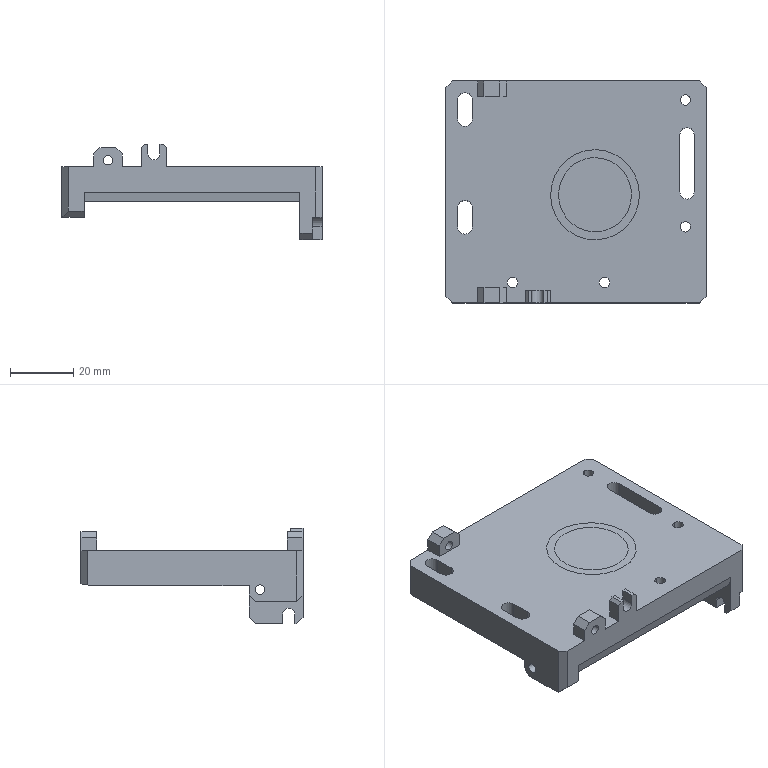NC program | NX | posted with a generic post | part box 82 x 70 x 30 mm
Whole program:
N10 G17 G21 G94 G90
(HOLE_MILLING , TOOL : D10)
N12 T10 M6
N14 G54
N16 G17 G0 G90 X34.989 Y6. B0. C0. S9500 M3
N18 G43 Z50. H10
N20 Z-1.904
N22 G94 G3 X37.177 Y8.188 R2.188 F1500.
N24 X34.989 Y10.375 R2.188
N26 X34.989 Y10.375 Z-2.404 I0. J-4.375
N28 X34.989 Y10.375 Z-2.904 I0. J-4.375
N30 X34.989 Y10.375 Z-3.404 I0. J-4.375
N32 X34.989 Y10.375 Z-3.904 I0. J-4.375
N34 X34.989 Y10.375 Z-4.404 I0. J-4.375
N36 X34.989 Y10.375 Z-4.904 I0. J-4.375
N38 X34.989 Y10.375 Z-5.404 I0. J-4.375
N40 X34.989 Y10.375 Z-5.904 I0. J-4.375
N42 X34.989 Y10.375 Z-6.404 I0. J-4.375
N44 X34.989 Y10.375 Z-6.904 I0. J-4.375
N46 X34.989 Y10.375 Z-7.404 I0. J-4.375
N48 X34.989 Y10.375 Z-7.904 I0. J-4.375
N50 X34.989 Y10.375 Z-8.404 I0. J-4.375
N52 X34.989 Y10.375 Z-8.904 I0. J-4.375
N54 X34.989 Y10.375 Z-9.404 I0. J-4.375
N56 X34.989 Y10.375 Z-9.904 I0. J-4.375
N58 X34.989 Y10.375 Z-10.404 I0. J-4.375
N60 X34.989 Y10.375 Z-10.904 I0. J-4.375
N62 X34.989 Y10.375 Z-11.404 I0. J-4.375
N64 X34.989 Y10.375 Z-11.904 I0. J-4.375
N66 X30.687 Y6.792 Z-12.015 R4.375
N68 X34.197 Y1.697 R4.375
N70 X30.687 Y6.792 R-4.375
N72 X32.442 Y4.245 R2.188
N74 X34.989 Y6. R2.188
N76 G0 Z-1.904
N78 G3 X39.364 Y10.375 R4.375
N80 X34.989 Y14.75 R4.375
N82 X34.989 Y14.75 Z-2.404 I0. J-8.75
N84 X34.989 Y14.75 Z-2.904 I0. J-8.75
N86 X34.989 Y14.75 Z-3.404 I0. J-8.75
N88 X34.989 Y14.75 Z-3.904 I0. J-8.75
N90 X34.989 Y14.75 Z-4.404 I0. J-8.75
N92 X34.989 Y14.75 Z-4.904 I0. J-8.75
N94 X34.989 Y14.75 Z-5.404 I0. J-8.75
N96 X34.989 Y14.75 Z-5.904 I0. J-8.75
N98 X34.989 Y14.75 Z-6.404 I0. J-8.75
N100 X34.989 Y14.75 Z-6.904 I0. J-8.75
N102 X34.989 Y14.75 Z-7.404 I0. J-8.75
N104 X34.989 Y14.75 Z-7.904 I0. J-8.75
N106 X34.989 Y14.75 Z-8.404 I0. J-8.75
N108 X34.989 Y14.75 Z-8.904 I0. J-8.75
N110 X34.989 Y14.75 Z-9.404 I0. J-8.75
N112 X34.989 Y14.75 Z-9.904 I0. J-8.75
N114 X34.989 Y14.75 Z-10.404 I0. J-8.75
N116 X34.989 Y14.75 Z-10.904 I0. J-8.75
N118 X34.989 Y14.75 Z-11.404 I0. J-8.75
N120 X34.989 Y14.75 Z-11.904 I0. J-8.75
N122 X26.384 Y7.584 Z-12.015 R8.75
N124 X33.405 Y-2.605 R8.75
N126 X26.384 Y7.584 R-8.75
N128 X29.894 Y2.49 R4.375
N130 X34.989 Y6. R4.375
N132 G0 Z50.
(HOLE_MILLING_COPY , TOOL : D10)
N134 Z-11.015
N136 G3 X36.864 Y7.875 R1.875
N138 X34.989 Y9.75 R1.875
N140 X34.989 Y9.75 Z-11.515 I0. J-3.75
N142 X34.989 Y9.75 Z-12.015 I0. J-3.75
N144 X34.989 Y9.75 Z-12.515 I0. J-3.75
N146 X34.989 Y9.75 Z-13.015 I0. J-3.75
N148 X34.989 Y9.75 Z-13.515 I0. J-3.75
N150 X31.239 Y6. R3.75
N152 X34.989 Y9.75 R-3.75
N154 X33.114 Y7.875 R1.875
N156 X34.989 Y6. R1.875
N158 G0 Z-11.015
N160 G3 X38.739 Y9.75 R3.75
N162 X34.989 Y13.5 R3.75
N164 X34.989 Y13.5 Z-11.515 I0. J-7.5
N166 X34.989 Y13.5 Z-12.015 I0. J-7.5
N168 X34.989 Y13.5 Z-12.515 I0. J-7.5
N170 X34.989 Y13.5 Z-13.015 I0. J-7.5
N172 X34.989 Y13.5 Z-13.515 I0. J-7.5
N174 X27.489 Y6. R7.5
N176 X34.989 Y13.5 R-7.5
N178 X31.239 Y9.75 R3.75
N180 X34.989 Y6. R3.75
N182 G0 Z50.
(HOLE_MILLING_COPY_COPY , TOOL : D10)
N184 Z-12.515
N186 G3 X36.614 Y7.625 R1.625
N188 X34.989 Y9.25 R1.625
N190 X34.989 Y9.25 Z-13.015 I0. J-3.25
N192 X34.989 Y9.25 Z-13.515 I0. J-3.25
N194 X34.989 Y9.25 Z-14.015 I0. J-3.25
N196 X34.989 Y9.25 Z-14.515 I0. J-3.25
N198 X34.989 Y9.25 Z-15.015 I0. J-3.25
N200 X34.989 Y9.25 Z-15.515 I0. J-3.25
N202 X34.989 Y9.25 Z-16.015 I0. J-3.25
N204 X34.989 Y9.25 Z-16.515 I0. J-3.25
N206 X34.989 Y9.25 Z-17.015 I0. J-3.25
N208 X34.989 Y9.25 Z-17.515 I0. J-3.25
N210 X34.989 Y9.25 Z-18.015 I0. J-3.25
N212 X34.989 Y9.25 Z-18.515 I0. J-3.25
N214 X34.989 Y9.25 Z-19.015 I0. J-3.25
N216 X34.989 Y9.25 Z-19.515 I0. J-3.25
N218 X32.901 Y8.491 Z-19.57 R3.25
N220 X32.499 Y3.912 R3.25
N222 X32.901 Y8.491 R-3.25
N224 X32.7 Y6.201 R1.625
N226 X34.989 Y6. R1.625
N228 G0 Z-12.515
N230 G3 X38.239 Y9.25 R3.25
N232 X34.989 Y12.5 R3.25
N234 X34.989 Y12.5 Z-13.015 I0. J-6.5
N236 X34.989 Y12.5 Z-13.515 I0. J-6.5
N238 X34.989 Y12.5 Z-14.015 I0. J-6.5
N240 X34.989 Y12.5 Z-14.515 I0. J-6.5
N242 X34.989 Y12.5 Z-15.015 I0. J-6.5
N244 X34.989 Y12.5 Z-15.515 I0. J-6.5
N246 X34.989 Y12.5 Z-16.015 I0. J-6.5
N248 X34.989 Y12.5 Z-16.515 I0. J-6.5
N250 X34.989 Y12.5 Z-17.015 I0. J-6.5
N252 X34.989 Y12.5 Z-17.515 I0. J-6.5
N254 X34.989 Y12.5 Z-18.015 I0. J-6.5
N256 X34.989 Y12.5 Z-18.515 I0. J-6.5
N258 X34.989 Y12.5 Z-19.015 I0. J-6.5
N260 X34.989 Y12.5 Z-19.515 I0. J-6.5
N262 X30.813 Y10.981 Z-19.57 R6.5
N264 X30.008 Y1.824 R6.5
N266 X30.813 Y10.981 R-6.5
N268 X30.411 Y6.403 R3.25
N270 X34.989 Y6. R3.25
N272 G0 Z50.
N274 M5
(PLANAR_MILL_1 , TOOL : T6H1)
N276 T08 M6
N278 G54
N280 G17 G0 G90 X27.836 Y8.567 B0. C0. S8000 M3
N282 G43 Z50. H8
N284 Z-9.015
N286 G94 G1 Z-12.015 F1250.
N288 X24.889 Y6.866
N290 G3 X24.389 Y6. R1.
N292 X34.989 Y-4.6 R10.6
N294 X24.389 Y6. R-10.6
N296 X24.889 Y5.134 R1.
N298 G1 X24.789 Y6.866
N300 G3 X24.289 Y6. R1.
N302 X34.989 Y-4.7 R10.7
N304 X24.289 Y6. R-10.7
N306 X24.789 Y5.134 R1.
N308 G1 X24.689 Y6.866
N310 G3 X24.189 Y6. R1.
N312 X34.989 Y-4.8 R10.8
N314 X24.189 Y6. R-10.8
N316 X24.689 Y5.134 R1.
N318 G1 X24.589 Y6.866
N320 G3 X24.089 Y6. R1.
N322 X34.989 Y-4.9 R10.9
N324 X24.089 Y6. R-10.9
N326 X24.589 Y5.134 R1.
N328 G1 X24.489 Y6.866
N330 G3 X23.989 Y6. R1.
N332 X34.989 Y-5. R11.
N334 X23.989 Y6. R-11.
N336 X24.489 Y5.134 R1.
N338 G1 X24.389 Y6.866
N340 G3 X23.889 Y6. R1.
N342 X34.989 Y-5.1 R11.1
N344 X23.889 Y6. R-11.1
N346 X24.389 Y5.134 R1.
N348 G1 X24.289 Y6.866
N350 G3 X23.789 Y6. R1.
N352 X34.989 Y-5.2 R11.2
N354 X23.789 Y6. R-11.2
N356 X24.289 Y5.134 R1.
N358 G1 X24.189 Y6.866
N360 G3 X23.689 Y6. R1.
N362 X34.989 Y-5.3 R11.3
N364 X23.689 Y6. R-11.3
N366 X24.189 Y5.134 R1.
N368 G1 X24.089 Y6.866
N370 G3 X23.589 Y6. R1.
N372 X34.989 Y-5.4 R11.4
N374 X23.589 Y6. R-11.4
N376 X24.089 Y5.134 R1.
N378 G1 X23.989 Y6.866
N380 G3 X23.489 Y6. R1.
N382 X34.989 Y-5.5 R11.5
N384 X23.489 Y6. R-11.5
N386 X23.989 Y5.134 R1.
N388 G1 X26.875 Y3.468
N390 Z-9.015
N392 G0 Z50.
N394 M5
(THREAD_MILLING , TOOL : D2.4XYD)
N396 T09 M6
N398 G54
N400 G17 G0 G90 X34.989 Y6. B0. C0. S7500 M3
N402 G43 Z50. H9
N404 Z-1.898
N406 G42 G94 G1 X34.311 Y18.031 F1250. D9
N408 G2 X34.989 Y18.633 Z-1.904 R0.683
N410 X34.989 Y18.633 Z-2.404 I0. J-12.633
N412 X34.989 Y18.633 Z-2.904 I0. J-12.633
N414 X34.989 Y18.633 Z-3.404 I0. J-12.633
N416 X34.989 Y18.633 Z-3.904 I0. J-12.633
N418 X34.989 Y18.633 Z-4.404 I0. J-12.633
N420 X34.989 Y18.633 Z-4.904 I0. J-12.633
N422 X34.989 Y18.633 Z-5.404 I0. J-12.633
N424 X34.989 Y18.633 Z-5.904 I0. J-12.633
N426 X34.989 Y18.633 Z-6.404 I0. J-12.633
N428 X34.989 Y18.633 Z-6.904 I0. J-12.633
N430 X34.989 Y18.633 Z-7.404 I0. J-12.633
N432 X34.989 Y18.633 Z-7.904 I0. J-12.633
N434 X34.989 Y18.633 Z-8.404 I0. J-12.633
N436 X34.989 Y18.633 Z-8.904 I0. J-12.633
N438 X34.989 Y18.633 Z-9.404 I0. J-12.633
N440 X34.989 Y18.633 Z-9.904 I0. J-12.633
N442 X34.989 Y18.633 Z-10.404 I0. J-12.633
N444 X34.989 Y18.633 Z-10.904 I0. J-12.633
N446 X47.414 Y8.288 Z-11.015 R12.633
N448 X46.944 Y7.512 Z-11.021 R0.683
N450 G40
N452 G1 X34.989 Y6.
N454 G0 Z-1.897
N456 G42 G1 X34.217 Y18.025
N458 G2 X34.989 Y18.717 Z-1.904 R0.777
N460 X34.989 Y18.717 Z-2.404 I0. J-12.717
N462 X34.989 Y18.717 Z-2.904 I0. J-12.717
N464 X34.989 Y18.717 Z-3.404 I0. J-12.717
N466 X34.989 Y18.717 Z-3.904 I0. J-12.717
N468 X34.989 Y18.717 Z-4.404 I0. J-12.717
N470 X34.989 Y18.717 Z-4.904 I0. J-12.717
N472 X34.989 Y18.717 Z-5.404 I0. J-12.717
N474 X34.989 Y18.717 Z-5.904 I0. J-12.717
N476 X34.989 Y18.717 Z-6.404 I0. J-12.717
N478 X34.989 Y18.717 Z-6.904 I0. J-12.717
N480 X34.989 Y18.717 Z-7.404 I0. J-12.717
N482 X34.989 Y18.717 Z-7.904 I0. J-12.717
N484 X34.989 Y18.717 Z-8.404 I0. J-12.717
N486 X34.989 Y18.717 Z-8.904 I0. J-12.717
N488 X34.989 Y18.717 Z-9.404 I0. J-12.717
N490 X34.989 Y18.717 Z-9.904 I0. J-12.717
N492 X34.989 Y18.717 Z-10.404 I0. J-12.717
N494 X34.989 Y18.717 Z-10.904 I0. J-12.717
N496 X47.496 Y8.303 Z-11.015 R12.717
N498 X46.955 Y7.418 Z-11.022 R0.777
N500 G40
N502 G1 X34.989 Y6.
N504 G0 Z-1.897
N506 G42 G1 X34.123 Y18.019
N508 G2 X34.989 Y18.8 Z-1.904 R0.87
N510 X34.989 Y18.8 Z-2.404 I0. J-12.8
N512 X34.989 Y18.8 Z-2.904 I0. J-12.8
N514 X34.989 Y18.8 Z-3.404 I0. J-12.8
N516 X34.989 Y18.8 Z-3.904 I0. J-12.8
N518 X34.989 Y18.8 Z-4.404 I0. J-12.8
N520 X34.989 Y18.8 Z-4.904 I0. J-12.8
N522 X34.989 Y18.8 Z-5.404 I0. J-12.8
N524 X34.989 Y18.8 Z-5.904 I0. J-12.8
N526 X34.989 Y18.8 Z-6.404 I0. J-12.8
N528 X34.989 Y18.8 Z-6.904 I0. J-12.8
N530 X34.989 Y18.8 Z-7.404 I0. J-12.8
N532 X34.989 Y18.8 Z-7.904 I0. J-12.8
N534 X34.989 Y18.8 Z-8.404 I0. J-12.8
N536 X34.989 Y18.8 Z-8.904 I0. J-12.8
N538 X34.989 Y18.8 Z-9.404 I0. J-12.8
N540 X34.989 Y18.8 Z-9.904 I0. J-12.8
N542 X34.989 Y18.8 Z-10.404 I0. J-12.8
N544 X34.989 Y18.8 Z-10.904 I0. J-12.8
N546 X47.578 Y8.318 Z-11.015 R12.8
N548 X46.966 Y7.325 Z-11.023 R0.87
N550 G40
N552 G1 X34.989 Y6.
N554 G0 Z50.
N556 M5
N558 M2